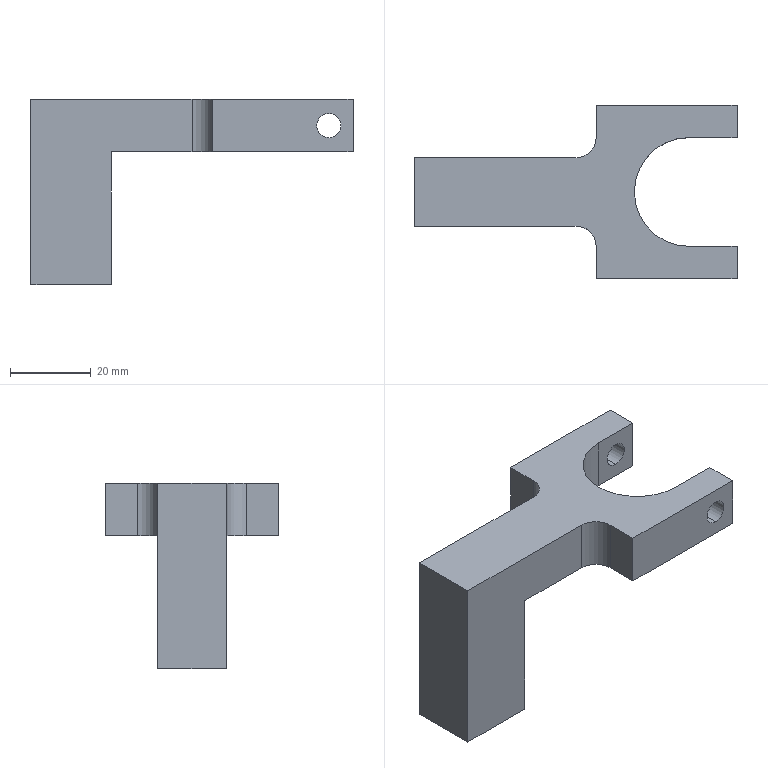Part | SolidWorks | features ICE 3, Extrusion 1, Fillet 1 | 1 solid | 23 faces | box 80 x 43 x 46 mm | volume 32483 mm3 | plane 15 | cylinder 8 | commonest cylinder face diameters 6 x4 10 x2 27 x2
STEP:
#1=CARTESIAN_POINT('',(6.,21.5,-3.));
#2=VERTEX_POINT('',#1);
#3=CARTESIAN_POINT('',(6.,21.5,3.));
#4=VERTEX_POINT('',#3);
#5=CARTESIAN_POINT('',(6.,21.5,0.));
#6=DIRECTION('',(0.,1.,0.));
#7=DIRECTION('',(0.,0.,-1.));
#8=AXIS2_PLACEMENT_3D('',#5,#6,#7);
#9=CIRCLE('',#8,3.);
#10=EDGE_CURVE('',#2,#4,#9,.T.);
#11=ORIENTED_EDGE('',*,*,#10,.T.);
#12=CARTESIAN_POINT('',(6.,13.5,3.));
#13=VERTEX_POINT('',#12);
#14=CARTESIAN_POINT('',(6.,29.985,3.));
#15=DIRECTION('',(0.,-1.,0.));
#16=VECTOR('',#15,1000.);
#17=LINE('',#14,#16);
#18=EDGE_CURVE('',#4,#13,#17,.T.);
#19=ORIENTED_EDGE('',*,*,#18,.T.);
#20=CARTESIAN_POINT('',(6.,13.5,-3.));
#21=VERTEX_POINT('',#20);
#22=CARTESIAN_POINT('',(6.,13.5,0.));
#23=DIRECTION('',(0.,1.,0.));
#24=DIRECTION('',(0.,0.,1.));
#25=AXIS2_PLACEMENT_3D('',#22,#23,#24);
#26=CIRCLE('',#25,3.);
#27=EDGE_CURVE('',#21,#13,#26,.T.);
#28=ORIENTED_EDGE('',*,*,#27,.F.);
#29=CARTESIAN_POINT('',(6.,29.985,-3.));
#30=DIRECTION('',(0.,-1.,0.));
#31=VECTOR('',#30,1000.);
#32=LINE('',#29,#31);
#33=EDGE_CURVE('',#2,#21,#32,.T.);
#34=ORIENTED_EDGE('',*,*,#33,.F.);
#35=EDGE_LOOP('',(#11,#19,#28,#34));
#36=FACE_OUTER_BOUND('',#35,.T.);
#37=CARTESIAN_POINT('',(6.,29.985,0.));
#38=DIRECTION('',(0.,-1.,0.));
#39=DIRECTION('',(0.,0.,-1.));
#40=AXIS2_PLACEMENT_3D('',#37,#38,#39);
#41=CYLINDRICAL_SURFACE('',#40,3.);
#42=ADVANCED_FACE('',(#36),#41,.F.);
#43=CARTESIAN_POINT('',(6.,-13.5,3.));
#44=VERTEX_POINT('',#43);
#45=CARTESIAN_POINT('',(6.,-13.5,-3.));
#46=VERTEX_POINT('',#45);
#47=CARTESIAN_POINT('',(6.,-13.5,0.));
#48=DIRECTION('',(0.,-1.,0.));
#49=DIRECTION('',(0.,0.,-1.));
#50=AXIS2_PLACEMENT_3D('',#47,#48,#49);
#51=CIRCLE('',#50,3.);
#52=EDGE_CURVE('',#44,#46,#51,.T.);
#53=ORIENTED_EDGE('',*,*,#52,.F.);
#54=CARTESIAN_POINT('',(6.,-21.5,3.));
#55=VERTEX_POINT('',#54);
#56=CARTESIAN_POINT('',(6.,29.985,3.));
#57=DIRECTION('',(0.,-1.,0.));
#58=VECTOR('',#57,1000.);
#59=LINE('',#56,#58);
#60=EDGE_CURVE('',#44,#55,#59,.T.);
#61=ORIENTED_EDGE('',*,*,#60,.T.);
#62=CARTESIAN_POINT('',(6.,-21.5,-3.));
#63=VERTEX_POINT('',#62);
#64=CARTESIAN_POINT('',(6.,-21.5,0.));
#65=DIRECTION('',(0.,-1.,0.));
#66=DIRECTION('',(0.,0.,-1.));
#67=AXIS2_PLACEMENT_3D('',#64,#65,#66);
#68=CIRCLE('',#67,3.);
#69=EDGE_CURVE('',#55,#63,#68,.T.);
#70=ORIENTED_EDGE('',*,*,#69,.T.);
#71=CARTESIAN_POINT('',(6.,29.985,-3.));
#72=DIRECTION('',(0.,-1.,0.));
#73=VECTOR('',#72,1000.);
#74=LINE('',#71,#73);
#75=EDGE_CURVE('',#46,#63,#74,.T.);
#76=ORIENTED_EDGE('',*,*,#75,.F.);
#77=EDGE_LOOP('',(#53,#61,#70,#76));
#78=FACE_OUTER_BOUND('',#77,.T.);
#79=CARTESIAN_POINT('',(6.,29.985,0.));
#80=DIRECTION('',(0.,-1.,0.));
#81=DIRECTION('',(0.,0.,-1.));
#82=AXIS2_PLACEMENT_3D('',#79,#80,#81);
#83=CYLINDRICAL_SURFACE('',#82,3.);
#84=ADVANCED_FACE('',(#78),#83,.F.);
#85=CARTESIAN_POINT('',(-13.5,0.,6.5));
#86=VERTEX_POINT('',#85);
#87=CARTESIAN_POINT('',(0.,13.5,6.5));
#88=VERTEX_POINT('',#87);
#89=CARTESIAN_POINT('',(0.,0.,6.5));
#90=DIRECTION('',(0.,0.,-1.));
#91=DIRECTION('',(1.,0.,0.));
#92=AXIS2_PLACEMENT_3D('',#89,#90,#91);
#93=CIRCLE('',#92,13.5);
#94=EDGE_CURVE('',#86,#88,#93,.T.);
#95=ORIENTED_EDGE('',*,*,#94,.F.);
#96=CARTESIAN_POINT('',(-13.5,0.,-6.5));
#97=VERTEX_POINT('',#96);
#98=CARTESIAN_POINT('',(-13.5,0.,6.5));
#99=DIRECTION('',(0.,0.,-1.));
#100=VECTOR('',#99,1000.);
#101=LINE('',#98,#100);
#102=EDGE_CURVE('',#86,#97,#101,.T.);
#103=ORIENTED_EDGE('',*,*,#102,.T.);
#104=CARTESIAN_POINT('',(0.,13.5,-6.5));
#105=VERTEX_POINT('',#104);
#106=CARTESIAN_POINT('',(0.,0.,-6.5));
#107=DIRECTION('',(0.,0.,-1.));
#108=DIRECTION('',(1.,0.,0.));
#109=AXIS2_PLACEMENT_3D('',#106,#107,#108);
#110=CIRCLE('',#109,13.5);
#111=EDGE_CURVE('',#97,#105,#110,.T.);
#112=ORIENTED_EDGE('',*,*,#111,.T.);
#113=CARTESIAN_POINT('',(0.,13.5,6.5));
#114=DIRECTION('',(0.,0.,-1.));
#115=VECTOR('',#114,1000.);
#116=LINE('',#113,#115);
#117=EDGE_CURVE('',#88,#105,#116,.T.);
#118=ORIENTED_EDGE('',*,*,#117,.F.);
#119=EDGE_LOOP('',(#95,#103,#112,#118));
#120=FACE_OUTER_BOUND('',#119,.T.);
#121=CARTESIAN_POINT('',(0.,0.,6.5));
#122=DIRECTION('',(0.,0.,-1.));
#123=DIRECTION('',(-1.,0.,0.));
#124=AXIS2_PLACEMENT_3D('',#121,#122,#123);
#125=CYLINDRICAL_SURFACE('',#124,13.5);
#126=ADVANCED_FACE('',(#120),#125,.F.);
#127=CARTESIAN_POINT('',(-48.,8.5,-6.5));
#128=VERTEX_POINT('',#127);
#129=CARTESIAN_POINT('',(-48.,-8.5,-6.5));
#130=VERTEX_POINT('',#129);
#131=CARTESIAN_POINT('',(-48.,-8.5,-6.5));
#132=DIRECTION('',(0.,-1.,0.));
#133=VECTOR('',#132,1000.);
#134=LINE('',#131,#133);
#135=EDGE_CURVE('',#128,#130,#134,.T.);
#136=ORIENTED_EDGE('',*,*,#135,.F.);
#137=CARTESIAN_POINT('',(-28.,8.5,-6.5));
#138=VERTEX_POINT('',#137);
#139=CARTESIAN_POINT('',(-68.,8.5,-6.5));
#140=DIRECTION('',(-1.,0.,0.));
#141=VECTOR('',#140,1000.);
#142=LINE('',#139,#141);
#143=EDGE_CURVE('',#138,#128,#142,.T.);
#144=ORIENTED_EDGE('',*,*,#143,.F.);
#145=CARTESIAN_POINT('',(-23.,13.5,-6.5));
#146=VERTEX_POINT('',#145);
#147=CARTESIAN_POINT('',(-28.,13.5,-6.5));
#148=DIRECTION('',(0.,0.,1.));
#149=DIRECTION('',(1.,0.,0.));
#150=AXIS2_PLACEMENT_3D('',#147,#148,#149);
#151=CIRCLE('',#150,5.);
#152=EDGE_CURVE('',#138,#146,#151,.T.);
#153=ORIENTED_EDGE('',*,*,#152,.T.);
#154=CARTESIAN_POINT('',(-23.,21.5,-6.5));
#155=VERTEX_POINT('',#154);
#156=CARTESIAN_POINT('',(-23.,21.5,-6.5));
#157=DIRECTION('',(0.,-1.,0.));
#158=VECTOR('',#157,1000.);
#159=LINE('',#156,#158);
#160=EDGE_CURVE('',#155,#146,#159,.T.);
#161=ORIENTED_EDGE('',*,*,#160,.F.);
#162=CARTESIAN_POINT('',(12.,21.5,-6.5));
#163=VERTEX_POINT('',#162);
#164=CARTESIAN_POINT('',(12.,21.5,-6.5));
#165=DIRECTION('',(-1.,0.,0.));
#166=VECTOR('',#165,1000.);
#167=LINE('',#164,#166);
#168=EDGE_CURVE('',#163,#155,#167,.T.);
#169=ORIENTED_EDGE('',*,*,#168,.F.);
#170=CARTESIAN_POINT('',(12.,13.5,-6.5));
#171=VERTEX_POINT('',#170);
#172=CARTESIAN_POINT('',(12.,13.5,-6.5));
#173=DIRECTION('',(0.,1.,0.));
#174=VECTOR('',#173,1000.);
#175=LINE('',#172,#174);
#176=EDGE_CURVE('',#171,#163,#175,.T.);
#177=ORIENTED_EDGE('',*,*,#176,.F.);
#178=CARTESIAN_POINT('',(0.,13.5,-6.5));
#179=DIRECTION('',(1.,0.,0.));
#180=VECTOR('',#179,1000.);
#181=LINE('',#178,#180);
#182=EDGE_CURVE('',#105,#171,#181,.T.);
#183=ORIENTED_EDGE('',*,*,#182,.F.);
#184=ORIENTED_EDGE('',*,*,#111,.F.);
#185=CARTESIAN_POINT('',(0.,-13.5,-6.5));
#186=VERTEX_POINT('',#185);
#187=CARTESIAN_POINT('',(0.,0.,-6.5));
#188=DIRECTION('',(0.,0.,-1.));
#189=DIRECTION('',(1.,0.,0.));
#190=AXIS2_PLACEMENT_3D('',#187,#188,#189);
#191=CIRCLE('',#190,13.5);
#192=EDGE_CURVE('',#186,#97,#191,.T.);
#193=ORIENTED_EDGE('',*,*,#192,.F.);
#194=CARTESIAN_POINT('',(12.,-13.5,-6.5));
#195=VERTEX_POINT('',#194);
#196=CARTESIAN_POINT('',(12.,-13.5,-6.5));
#197=DIRECTION('',(-1.,0.,0.));
#198=VECTOR('',#197,1000.);
#199=LINE('',#196,#198);
#200=EDGE_CURVE('',#195,#186,#199,.T.);
#201=ORIENTED_EDGE('',*,*,#200,.F.);
#202=CARTESIAN_POINT('',(12.,-21.5,-6.5));
#203=VERTEX_POINT('',#202);
#204=CARTESIAN_POINT('',(12.,-21.5,-6.5));
#205=DIRECTION('',(0.,1.,0.));
#206=VECTOR('',#205,1000.);
#207=LINE('',#204,#206);
#208=EDGE_CURVE('',#203,#195,#207,.T.);
#209=ORIENTED_EDGE('',*,*,#208,.F.);
#210=CARTESIAN_POINT('',(-23.,-21.5,-6.5));
#211=VERTEX_POINT('',#210);
#212=CARTESIAN_POINT('',(-68.,-21.5,-6.5));
#213=DIRECTION('',(1.,0.,0.));
#214=VECTOR('',#213,1000.);
#215=LINE('',#212,#214);
#216=EDGE_CURVE('',#211,#203,#215,.T.);
#217=ORIENTED_EDGE('',*,*,#216,.F.);
#218=CARTESIAN_POINT('',(-23.,-13.5,-6.5));
#219=VERTEX_POINT('',#218);
#220=CARTESIAN_POINT('',(-23.,-21.5,-6.5));
#221=DIRECTION('',(0.,-1.,0.));
#222=VECTOR('',#221,1000.);
#223=LINE('',#220,#222);
#224=EDGE_CURVE('',#219,#211,#223,.T.);
#225=ORIENTED_EDGE('',*,*,#224,.F.);
#226=CARTESIAN_POINT('',(-28.,-8.5,-6.5));
#227=VERTEX_POINT('',#226);
#228=CARTESIAN_POINT('',(-28.,-13.5,-6.5));
#229=DIRECTION('',(0.,0.,1.));
#230=DIRECTION('',(1.,0.,0.));
#231=AXIS2_PLACEMENT_3D('',#228,#229,#230);
#232=CIRCLE('',#231,5.);
#233=EDGE_CURVE('',#219,#227,#232,.T.);
#234=ORIENTED_EDGE('',*,*,#233,.T.);
#235=CARTESIAN_POINT('',(-68.,-8.5,-6.5));
#236=DIRECTION('',(1.,0.,0.));
#237=VECTOR('',#236,1000.);
#238=LINE('',#235,#237);
#239=EDGE_CURVE('',#130,#227,#238,.T.);
#240=ORIENTED_EDGE('',*,*,#239,.F.);
#241=EDGE_LOOP('',(#136,#144,#153,#161,#169,#177,#183,#184,#193,#201,#209,#217,#225,#234,#240));
#242=FACE_OUTER_BOUND('',#241,.T.);
#243=CARTESIAN_POINT('',(0.,0.,-6.5));
#244=DIRECTION('',(0.,0.,1.));
#245=DIRECTION('',(1.,0.,0.));
#246=AXIS2_PLACEMENT_3D('',#243,#244,#245);
#247=PLANE('',#246);
#248=ADVANCED_FACE('',(#242),#247,.F.);
#249=ORIENTED_EDGE('',*,*,#102,.F.);
#250=CARTESIAN_POINT('',(0.,-13.5,6.5));
#251=VERTEX_POINT('',#250);
#252=CARTESIAN_POINT('',(0.,0.,6.5));
#253=DIRECTION('',(0.,0.,-1.));
#254=DIRECTION('',(1.,0.,0.));
#255=AXIS2_PLACEMENT_3D('',#252,#253,#254);
#256=CIRCLE('',#255,13.5);
#257=EDGE_CURVE('',#251,#86,#256,.T.);
#258=ORIENTED_EDGE('',*,*,#257,.F.);
#259=CARTESIAN_POINT('',(0.,-13.5,6.5));
#260=DIRECTION('',(0.,0.,-1.));
#261=VECTOR('',#260,1000.);
#262=LINE('',#259,#261);
#263=EDGE_CURVE('',#251,#186,#262,.T.);
#264=ORIENTED_EDGE('',*,*,#263,.T.);
#265=ORIENTED_EDGE('',*,*,#192,.T.);
#266=EDGE_LOOP('',(#249,#258,#264,#265));
#267=FACE_OUTER_BOUND('',#266,.T.);
#268=CARTESIAN_POINT('',(0.,0.,6.5));
#269=DIRECTION('',(0.,0.,-1.));
#270=DIRECTION('',(-1.,0.,0.));
#271=AXIS2_PLACEMENT_3D('',#268,#269,#270);
#272=CYLINDRICAL_SURFACE('',#271,13.5);
#273=ADVANCED_FACE('',(#267),#272,.F.);
#274=ORIENTED_EDGE('',*,*,#27,.T.);
#275=CARTESIAN_POINT('',(6.,13.5,0.));
#276=DIRECTION('',(0.,1.,0.));
#277=DIRECTION('',(0.,0.,1.));
#278=AXIS2_PLACEMENT_3D('',#275,#276,#277);
#279=CIRCLE('',#278,3.);
#280=EDGE_CURVE('',#13,#21,#279,.T.);
#281=ORIENTED_EDGE('',*,*,#280,.T.);
#282=EDGE_LOOP('',(#274,#281));
#283=FACE_BOUND('',#282,.T.);
#284=ORIENTED_EDGE('',*,*,#182,.T.);
#285=CARTESIAN_POINT('',(12.,13.5,6.5));
#286=VERTEX_POINT('',#285);
#287=CARTESIAN_POINT('',(12.,13.5,6.5));
#288=DIRECTION('',(0.,0.,-1.));
#289=VECTOR('',#288,1000.);
#290=LINE('',#287,#289);
#291=EDGE_CURVE('',#286,#171,#290,.T.);
#292=ORIENTED_EDGE('',*,*,#291,.F.);
#293=CARTESIAN_POINT('',(0.,13.5,6.5));
#294=DIRECTION('',(1.,0.,0.));
#295=VECTOR('',#294,1000.);
#296=LINE('',#293,#295);
#297=EDGE_CURVE('',#88,#286,#296,.T.);
#298=ORIENTED_EDGE('',*,*,#297,.F.);
#299=ORIENTED_EDGE('',*,*,#117,.T.);
#300=EDGE_LOOP('',(#284,#292,#298,#299));
#301=FACE_OUTER_BOUND('',#300,.T.);
#302=CARTESIAN_POINT('',(0.,13.5,6.5));
#303=DIRECTION('',(0.,1.,0.));
#304=DIRECTION('',(0.,0.,1.));
#305=AXIS2_PLACEMENT_3D('',#302,#303,#304);
#306=PLANE('',#305);
#307=ADVANCED_FACE('',(#283,#301),#306,.F.);
#308=ORIENTED_EDGE('',*,*,#176,.T.);
#309=CARTESIAN_POINT('',(12.,21.5,6.5));
#310=VERTEX_POINT('',#309);
#311=CARTESIAN_POINT('',(12.,21.5,6.5));
#312=DIRECTION('',(0.,0.,-1.));
#313=VECTOR('',#312,1000.);
#314=LINE('',#311,#313);
#315=EDGE_CURVE('',#310,#163,#314,.T.);
#316=ORIENTED_EDGE('',*,*,#315,.F.);
#317=CARTESIAN_POINT('',(12.,13.5,6.5));
#318=DIRECTION('',(0.,1.,0.));
#319=VECTOR('',#318,1000.);
#320=LINE('',#317,#319);
#321=EDGE_CURVE('',#286,#310,#320,.T.);
#322=ORIENTED_EDGE('',*,*,#321,.F.);
#323=ORIENTED_EDGE('',*,*,#291,.T.);
#324=EDGE_LOOP('',(#308,#316,#322,#323));
#325=FACE_OUTER_BOUND('',#324,.T.);
#326=CARTESIAN_POINT('',(12.,13.5,6.5));
#327=DIRECTION('',(-1.,0.,0.));
#328=DIRECTION('',(0.,0.,1.));
#329=AXIS2_PLACEMENT_3D('',#326,#327,#328);
#330=PLANE('',#329);
#331=ADVANCED_FACE('',(#325),#330,.F.);
#332=ORIENTED_EDGE('',*,*,#10,.F.);
#333=CARTESIAN_POINT('',(6.,21.5,0.));
#334=DIRECTION('',(0.,1.,0.));
#335=DIRECTION('',(0.,0.,-1.));
#336=AXIS2_PLACEMENT_3D('',#333,#334,#335);
#337=CIRCLE('',#336,3.);
#338=EDGE_CURVE('',#4,#2,#337,.T.);
#339=ORIENTED_EDGE('',*,*,#338,.F.);
#340=EDGE_LOOP('',(#332,#339));
#341=FACE_BOUND('',#340,.T.);
#342=ORIENTED_EDGE('',*,*,#168,.T.);
#343=CARTESIAN_POINT('',(-23.,21.5,6.5));
#344=VERTEX_POINT('',#343);
#345=CARTESIAN_POINT('',(-23.,21.5,-6.501));
#346=DIRECTION('',(0.,0.,1.));
#347=VECTOR('',#346,1000.);
#348=LINE('',#345,#347);
#349=EDGE_CURVE('',#155,#344,#348,.T.);
#350=ORIENTED_EDGE('',*,*,#349,.T.);
#351=CARTESIAN_POINT('',(12.,21.5,6.5));
#352=DIRECTION('',(-1.,0.,0.));
#353=VECTOR('',#352,1000.);
#354=LINE('',#351,#353);
#355=EDGE_CURVE('',#310,#344,#354,.T.);
#356=ORIENTED_EDGE('',*,*,#355,.F.);
#357=ORIENTED_EDGE('',*,*,#315,.T.);
#358=EDGE_LOOP('',(#342,#350,#356,#357));
#359=FACE_OUTER_BOUND('',#358,.T.);
#360=CARTESIAN_POINT('',(12.,21.5,6.5));
#361=DIRECTION('',(0.,-1.,0.));
#362=DIRECTION('',(0.,0.,-1.));
#363=AXIS2_PLACEMENT_3D('',#360,#361,#362);
#364=PLANE('',#363);
#365=ADVANCED_FACE('',(#341,#359),#364,.F.);
#366=CARTESIAN_POINT('',(-68.,8.5,6.5));
#367=VERTEX_POINT('',#366);
#368=CARTESIAN_POINT('',(-68.,-8.5,6.5));
#369=VERTEX_POINT('',#368);
#370=CARTESIAN_POINT('',(-68.,21.5,6.5));
#371=DIRECTION('',(0.,-1.,0.));
#372=VECTOR('',#371,1000.);
#373=LINE('',#370,#372);
#374=EDGE_CURVE('',#367,#369,#373,.T.);
#375=ORIENTED_EDGE('',*,*,#374,.F.);
#376=CARTESIAN_POINT('',(-68.,8.5,-39.5));
#377=VERTEX_POINT('',#376);
#378=CARTESIAN_POINT('',(-68.,8.5,-6.501));
#379=DIRECTION('',(0.,0.,1.));
#380=VECTOR('',#379,1000.);
#381=LINE('',#378,#380);
#382=EDGE_CURVE('',#377,#367,#381,.T.);
#383=ORIENTED_EDGE('',*,*,#382,.F.);
#384=CARTESIAN_POINT('',(-68.,-8.5,-39.5));
#385=VERTEX_POINT('',#384);
#386=CARTESIAN_POINT('',(-68.,-8.5,-39.5));
#387=DIRECTION('',(0.,1.,0.));
#388=VECTOR('',#387,1000.);
#389=LINE('',#386,#388);
#390=EDGE_CURVE('',#385,#377,#389,.T.);
#391=ORIENTED_EDGE('',*,*,#390,.F.);
#392=CARTESIAN_POINT('',(-68.,-8.5,-6.501));
#393=DIRECTION('',(0.,0.,1.));
#394=VECTOR('',#393,1000.);
#395=LINE('',#392,#394);
#396=EDGE_CURVE('',#385,#369,#395,.T.);
#397=ORIENTED_EDGE('',*,*,#396,.T.);
#398=EDGE_LOOP('',(#375,#383,#391,#397));
#399=FACE_OUTER_BOUND('',#398,.T.);
#400=CARTESIAN_POINT('',(-68.,21.5,6.5));
#401=DIRECTION('',(1.,0.,0.));
#402=DIRECTION('',(0.,0.,-1.));
#403=AXIS2_PLACEMENT_3D('',#400,#401,#402);
#404=PLANE('',#403);
#405=ADVANCED_FACE('',(#399),#404,.F.);
#406=CARTESIAN_POINT('',(6.,-21.5,0.));
#407=DIRECTION('',(0.,-1.,0.));
#408=DIRECTION('',(0.,0.,-1.));
#409=AXIS2_PLACEMENT_3D('',#406,#407,#408);
#410=CIRCLE('',#409,3.);
#411=EDGE_CURVE('',#63,#55,#410,.T.);
#412=ORIENTED_EDGE('',*,*,#411,.F.);
#413=ORIENTED_EDGE('',*,*,#69,.F.);
#414=EDGE_LOOP('',(#412,#413));
#415=FACE_BOUND('',#414,.T.);
#416=CARTESIAN_POINT('',(-23.,-21.5,6.5));
#417=VERTEX_POINT('',#416);
#418=CARTESIAN_POINT('',(12.,-21.5,6.5));
#419=VERTEX_POINT('',#418);
#420=CARTESIAN_POINT('',(-68.,-21.5,6.5));
#421=DIRECTION('',(1.,0.,0.));
#422=VECTOR('',#421,1000.);
#423=LINE('',#420,#422);
#424=EDGE_CURVE('',#417,#419,#423,.T.);
#425=ORIENTED_EDGE('',*,*,#424,.F.);
#426=CARTESIAN_POINT('',(-23.,-21.5,-6.501));
#427=DIRECTION('',(0.,0.,1.));
#428=VECTOR('',#427,1000.);
#429=LINE('',#426,#428);
#430=EDGE_CURVE('',#211,#417,#429,.T.);
#431=ORIENTED_EDGE('',*,*,#430,.F.);
#432=ORIENTED_EDGE('',*,*,#216,.T.);
#433=CARTESIAN_POINT('',(12.,-21.5,6.5));
#434=DIRECTION('',(0.,0.,-1.));
#435=VECTOR('',#434,1000.);
#436=LINE('',#433,#435);
#437=EDGE_CURVE('',#419,#203,#436,.T.);
#438=ORIENTED_EDGE('',*,*,#437,.F.);
#439=EDGE_LOOP('',(#425,#431,#432,#438));
#440=FACE_OUTER_BOUND('',#439,.T.);
#441=CARTESIAN_POINT('',(-68.,-21.5,6.5));
#442=DIRECTION('',(0.,1.,0.));
#443=DIRECTION('',(0.,0.,1.));
#444=AXIS2_PLACEMENT_3D('',#441,#442,#443);
#445=PLANE('',#444);
#446=ADVANCED_FACE('',(#415,#440),#445,.F.);
#447=ORIENTED_EDGE('',*,*,#208,.T.);
#448=CARTESIAN_POINT('',(12.,-13.5,6.5));
#449=VERTEX_POINT('',#448);
#450=CARTESIAN_POINT('',(12.,-13.5,6.5));
#451=DIRECTION('',(0.,0.,-1.));
#452=VECTOR('',#451,1000.);
#453=LINE('',#450,#452);
#454=EDGE_CURVE('',#449,#195,#453,.T.);
#455=ORIENTED_EDGE('',*,*,#454,.F.);
#456=CARTESIAN_POINT('',(12.,-21.5,6.5));
#457=DIRECTION('',(0.,1.,0.));
#458=VECTOR('',#457,1000.);
#459=LINE('',#456,#458);
#460=EDGE_CURVE('',#419,#449,#459,.T.);
#461=ORIENTED_EDGE('',*,*,#460,.F.);
#462=ORIENTED_EDGE('',*,*,#437,.T.);
#463=EDGE_LOOP('',(#447,#455,#461,#462));
#464=FACE_OUTER_BOUND('',#463,.T.);
#465=CARTESIAN_POINT('',(12.,-21.5,6.5));
#466=DIRECTION('',(-1.,0.,0.));
#467=DIRECTION('',(0.,0.,1.));
#468=AXIS2_PLACEMENT_3D('',#465,#466,#467);
#469=PLANE('',#468);
#470=ADVANCED_FACE('',(#464),#469,.F.);
#471=CARTESIAN_POINT('',(6.,-13.5,0.));
#472=DIRECTION('',(0.,-1.,0.));
#473=DIRECTION('',(0.,0.,-1.));
#474=AXIS2_PLACEMENT_3D('',#471,#472,#473);
#475=CIRCLE('',#474,3.);
#476=EDGE_CURVE('',#46,#44,#475,.T.);
#477=ORIENTED_EDGE('',*,*,#476,.T.);
#478=ORIENTED_EDGE('',*,*,#52,.T.);
#479=EDGE_LOOP('',(#477,#478));
#480=FACE_BOUND('',#479,.T.);
#481=ORIENTED_EDGE('',*,*,#200,.T.);
#482=ORIENTED_EDGE('',*,*,#263,.F.);
#483=CARTESIAN_POINT('',(12.,-13.5,6.5));
#484=DIRECTION('',(-1.,0.,0.));
#485=VECTOR('',#484,1000.);
#486=LINE('',#483,#485);
#487=EDGE_CURVE('',#449,#251,#486,.T.);
#488=ORIENTED_EDGE('',*,*,#487,.F.);
#489=ORIENTED_EDGE('',*,*,#454,.T.);
#490=EDGE_LOOP('',(#481,#482,#488,#489));
#491=FACE_OUTER_BOUND('',#490,.T.);
#492=CARTESIAN_POINT('',(12.,-13.5,6.5));
#493=DIRECTION('',(0.,-1.,0.));
#494=DIRECTION('',(0.,0.,-1.));
#495=AXIS2_PLACEMENT_3D('',#492,#493,#494);
#496=PLANE('',#495);
#497=ADVANCED_FACE('',(#480,#491),#496,.F.);
#498=CARTESIAN_POINT('',(-23.,13.5,6.5));
#499=VERTEX_POINT('',#498);
#500=CARTESIAN_POINT('',(-23.,21.5,6.5));
#501=DIRECTION('',(0.,1.,0.));
#502=VECTOR('',#501,1000.);
#503=LINE('',#500,#502);
#504=EDGE_CURVE('',#499,#344,#503,.T.);
#505=ORIENTED_EDGE('',*,*,#504,.F.);
#506=CARTESIAN_POINT('',(-28.,8.5,6.5));
#507=VERTEX_POINT('',#506);
#508=CARTESIAN_POINT('',(-28.,13.5,6.5));
#509=DIRECTION('',(0.,0.,-1.));
#510=DIRECTION('',(1.,0.,0.));
#511=AXIS2_PLACEMENT_3D('',#508,#509,#510);
#512=CIRCLE('',#511,5.);
#513=EDGE_CURVE('',#499,#507,#512,.T.);
#514=ORIENTED_EDGE('',*,*,#513,.T.);
#515=CARTESIAN_POINT('',(-68.,8.5,6.5));
#516=DIRECTION('',(1.,0.,0.));
#517=VECTOR('',#516,1000.);
#518=LINE('',#515,#517);
#519=EDGE_CURVE('',#367,#507,#518,.T.);
#520=ORIENTED_EDGE('',*,*,#519,.F.);
#521=ORIENTED_EDGE('',*,*,#374,.T.);
#522=CARTESIAN_POINT('',(-28.,-8.5,6.5));
#523=VERTEX_POINT('',#522);
#524=CARTESIAN_POINT('',(-68.,-8.5,6.5));
#525=DIRECTION('',(-1.,0.,0.));
#526=VECTOR('',#525,1000.);
#527=LINE('',#524,#526);
#528=EDGE_CURVE('',#523,#369,#527,.T.);
#529=ORIENTED_EDGE('',*,*,#528,.F.);
#530=CARTESIAN_POINT('',(-23.,-13.5,6.5));
#531=VERTEX_POINT('',#530);
#532=CARTESIAN_POINT('',(-28.,-13.5,6.5));
#533=DIRECTION('',(0.,0.,-1.));
#534=DIRECTION('',(1.,0.,0.));
#535=AXIS2_PLACEMENT_3D('',#532,#533,#534);
#536=CIRCLE('',#535,5.);
#537=EDGE_CURVE('',#523,#531,#536,.T.);
#538=ORIENTED_EDGE('',*,*,#537,.T.);
#539=CARTESIAN_POINT('',(-23.,-21.5,6.5));
#540=DIRECTION('',(0.,1.,0.));
#541=VECTOR('',#540,1000.);
#542=LINE('',#539,#541);
#543=EDGE_CURVE('',#417,#531,#542,.T.);
#544=ORIENTED_EDGE('',*,*,#543,.F.);
#545=ORIENTED_EDGE('',*,*,#424,.T.);
#546=ORIENTED_EDGE('',*,*,#460,.T.);
#547=ORIENTED_EDGE('',*,*,#487,.T.);
#548=ORIENTED_EDGE('',*,*,#257,.T.);
#549=ORIENTED_EDGE('',*,*,#94,.T.);
#550=ORIENTED_EDGE('',*,*,#297,.T.);
#551=ORIENTED_EDGE('',*,*,#321,.T.);
#552=ORIENTED_EDGE('',*,*,#355,.T.);
#553=EDGE_LOOP('',(#505,#514,#520,#521,#529,#538,#544,#545,#546,#547,#548,#549,#550,#551,#552));
#554=FACE_OUTER_BOUND('',#553,.T.);
#555=CARTESIAN_POINT('',(0.,0.,6.5));
#556=DIRECTION('',(0.,0.,1.));
#557=DIRECTION('',(1.,0.,0.));
#558=AXIS2_PLACEMENT_3D('',#555,#556,#557);
#559=PLANE('',#558);
#560=ADVANCED_FACE('',(#554),#559,.T.);
#561=ORIENTED_EDGE('',*,*,#396,.F.);
#562=CARTESIAN_POINT('',(-48.,-8.5,-39.5));
#563=VERTEX_POINT('',#562);
#564=CARTESIAN_POINT('',(-68.,-8.5,-39.5));
#565=DIRECTION('',(-1.,0.,0.));
#566=VECTOR('',#565,1000.);
#567=LINE('',#564,#566);
#568=EDGE_CURVE('',#563,#385,#567,.T.);
#569=ORIENTED_EDGE('',*,*,#568,.F.);
#570=CARTESIAN_POINT('',(-48.,-8.5,-39.5));
#571=DIRECTION('',(0.,0.,1.));
#572=VECTOR('',#571,1000.);
#573=LINE('',#570,#572);
#574=EDGE_CURVE('',#563,#130,#573,.T.);
#575=ORIENTED_EDGE('',*,*,#574,.T.);
#576=ORIENTED_EDGE('',*,*,#239,.T.);
#577=CARTESIAN_POINT('',(-28.,-8.5,6.5));
#578=DIRECTION('',(0.,0.,1.));
#579=VECTOR('',#578,1000.);
#580=LINE('',#577,#579);
#581=EDGE_CURVE('',#227,#523,#580,.T.);
#582=ORIENTED_EDGE('',*,*,#581,.T.);
#583=ORIENTED_EDGE('',*,*,#528,.T.);
#584=EDGE_LOOP('',(#561,#569,#575,#576,#582,#583));
#585=FACE_OUTER_BOUND('',#584,.T.);
#586=CARTESIAN_POINT('',(-68.,-8.5,-6.501));
#587=DIRECTION('',(0.,1.,0.));
#588=DIRECTION('',(0.,0.,1.));
#589=AXIS2_PLACEMENT_3D('',#586,#587,#588);
#590=PLANE('',#589);
#591=ADVANCED_FACE('',(#585),#590,.F.);
#592=ORIENTED_EDGE('',*,*,#543,.T.);
#593=CARTESIAN_POINT('',(-23.,-13.5,-6.5));
#594=DIRECTION('',(0.,0.,-1.));
#595=VECTOR('',#594,1000.);
#596=LINE('',#593,#595);
#597=EDGE_CURVE('',#531,#219,#596,.T.);
#598=ORIENTED_EDGE('',*,*,#597,.T.);
#599=ORIENTED_EDGE('',*,*,#224,.T.);
#600=ORIENTED_EDGE('',*,*,#430,.T.);
#601=EDGE_LOOP('',(#592,#598,#599,#600));
#602=FACE_OUTER_BOUND('',#601,.T.);
#603=CARTESIAN_POINT('',(-23.,-21.5,-6.501));
#604=DIRECTION('',(1.,0.,0.));
#605=DIRECTION('',(0.,0.,-1.));
#606=AXIS2_PLACEMENT_3D('',#603,#604,#605);
#607=PLANE('',#606);
#608=ADVANCED_FACE('',(#602),#607,.F.);
#609=ORIENTED_EDGE('',*,*,#160,.T.);
#610=CARTESIAN_POINT('',(-23.,13.5,6.5));
#611=DIRECTION('',(0.,0.,1.));
#612=VECTOR('',#611,1000.);
#613=LINE('',#610,#612);
#614=EDGE_CURVE('',#146,#499,#613,.T.);
#615=ORIENTED_EDGE('',*,*,#614,.T.);
#616=ORIENTED_EDGE('',*,*,#504,.T.);
#617=ORIENTED_EDGE('',*,*,#349,.F.);
#618=EDGE_LOOP('',(#609,#615,#616,#617));
#619=FACE_OUTER_BOUND('',#618,.T.);
#620=CARTESIAN_POINT('',(-23.,21.5,-6.501));
#621=DIRECTION('',(1.,0.,0.));
#622=DIRECTION('',(0.,0.,-1.));
#623=AXIS2_PLACEMENT_3D('',#620,#621,#622);
#624=PLANE('',#623);
#625=ADVANCED_FACE('',(#619),#624,.F.);
#626=ORIENTED_EDGE('',*,*,#519,.T.);
#627=CARTESIAN_POINT('',(-28.,8.5,-6.5));
#628=DIRECTION('',(0.,0.,-1.));
#629=VECTOR('',#628,1000.);
#630=LINE('',#627,#629);
#631=EDGE_CURVE('',#507,#138,#630,.T.);
#632=ORIENTED_EDGE('',*,*,#631,.T.);
#633=ORIENTED_EDGE('',*,*,#143,.T.);
#634=CARTESIAN_POINT('',(-48.,8.5,-39.5));
#635=VERTEX_POINT('',#634);
#636=CARTESIAN_POINT('',(-48.,8.5,-39.5));
#637=DIRECTION('',(0.,0.,1.));
#638=VECTOR('',#637,1000.);
#639=LINE('',#636,#638);
#640=EDGE_CURVE('',#635,#128,#639,.T.);
#641=ORIENTED_EDGE('',*,*,#640,.F.);
#642=CARTESIAN_POINT('',(-68.,8.5,-39.5));
#643=DIRECTION('',(1.,0.,0.));
#644=VECTOR('',#643,1000.);
#645=LINE('',#642,#644);
#646=EDGE_CURVE('',#377,#635,#645,.T.);
#647=ORIENTED_EDGE('',*,*,#646,.F.);
#648=ORIENTED_EDGE('',*,*,#382,.T.);
#649=EDGE_LOOP('',(#626,#632,#633,#641,#647,#648));
#650=FACE_OUTER_BOUND('',#649,.T.);
#651=CARTESIAN_POINT('',(-68.,8.5,-6.501));
#652=DIRECTION('',(0.,-1.,0.));
#653=DIRECTION('',(0.,0.,-1.));
#654=AXIS2_PLACEMENT_3D('',#651,#652,#653);
#655=PLANE('',#654);
#656=ADVANCED_FACE('',(#650),#655,.F.);
#657=ORIENTED_EDGE('',*,*,#233,.F.);
#658=ORIENTED_EDGE('',*,*,#597,.F.);
#659=ORIENTED_EDGE('',*,*,#537,.F.);
#660=ORIENTED_EDGE('',*,*,#581,.F.);
#661=EDGE_LOOP('',(#657,#658,#659,#660));
#662=FACE_OUTER_BOUND('',#661,.T.);
#663=CARTESIAN_POINT('',(-28.,-13.5,-6.501));
#664=DIRECTION('',(0.,0.,-1.));
#665=DIRECTION('',(-1.,0.,0.));
#666=AXIS2_PLACEMENT_3D('',#663,#664,#665);
#667=CYLINDRICAL_SURFACE('',#666,5.);
#668=ADVANCED_FACE('',(#662),#667,.F.);
#669=ORIENTED_EDGE('',*,*,#152,.F.);
#670=ORIENTED_EDGE('',*,*,#631,.F.);
#671=ORIENTED_EDGE('',*,*,#513,.F.);
#672=ORIENTED_EDGE('',*,*,#614,.F.);
#673=EDGE_LOOP('',(#669,#670,#671,#672));
#674=FACE_OUTER_BOUND('',#673,.T.);
#675=CARTESIAN_POINT('',(-28.,13.5,-6.501));
#676=DIRECTION('',(0.,0.,-1.));
#677=DIRECTION('',(-1.,0.,0.));
#678=AXIS2_PLACEMENT_3D('',#675,#676,#677);
#679=CYLINDRICAL_SURFACE('',#678,5.);
#680=ADVANCED_FACE('',(#674),#679,.F.);
#681=ORIENTED_EDGE('',*,*,#135,.T.);
#682=ORIENTED_EDGE('',*,*,#574,.F.);
#683=CARTESIAN_POINT('',(-48.,-8.5,-39.5));
#684=DIRECTION('',(0.,-1.,0.));
#685=VECTOR('',#684,1000.);
#686=LINE('',#683,#685);
#687=EDGE_CURVE('',#635,#563,#686,.T.);
#688=ORIENTED_EDGE('',*,*,#687,.F.);
#689=ORIENTED_EDGE('',*,*,#640,.T.);
#690=EDGE_LOOP('',(#681,#682,#688,#689));
#691=FACE_OUTER_BOUND('',#690,.T.);
#692=CARTESIAN_POINT('',(-48.,-8.5,-39.5));
#693=DIRECTION('',(-1.,0.,0.));
#694=DIRECTION('',(0.,0.,1.));
#695=AXIS2_PLACEMENT_3D('',#692,#693,#694);
#696=PLANE('',#695);
#697=ADVANCED_FACE('',(#691),#696,.F.);
#698=ORIENTED_EDGE('',*,*,#390,.T.);
#699=ORIENTED_EDGE('',*,*,#646,.T.);
#700=ORIENTED_EDGE('',*,*,#687,.T.);
#701=ORIENTED_EDGE('',*,*,#568,.T.);
#702=EDGE_LOOP('',(#698,#699,#700,#701));
#703=FACE_OUTER_BOUND('',#702,.T.);
#704=CARTESIAN_POINT('',(0.,0.,-39.5));
#705=DIRECTION('',(0.,0.,-1.));
#706=DIRECTION('',(-1.,0.,0.));
#707=AXIS2_PLACEMENT_3D('',#704,#705,#706);
#708=PLANE('',#707);
#709=ADVANCED_FACE('',(#703),#708,.T.);
#710=ORIENTED_EDGE('',*,*,#60,.F.);
#711=ORIENTED_EDGE('',*,*,#476,.F.);
#712=ORIENTED_EDGE('',*,*,#75,.T.);
#713=ORIENTED_EDGE('',*,*,#411,.T.);
#714=EDGE_LOOP('',(#710,#711,#712,#713));
#715=FACE_OUTER_BOUND('',#714,.T.);
#716=CARTESIAN_POINT('',(6.,29.985,0.));
#717=DIRECTION('',(0.,-1.,0.));
#718=DIRECTION('',(0.,0.,-1.));
#719=AXIS2_PLACEMENT_3D('',#716,#717,#718);
#720=CYLINDRICAL_SURFACE('',#719,3.);
#721=ADVANCED_FACE('',(#715),#720,.F.);
#722=ORIENTED_EDGE('',*,*,#18,.F.);
#723=ORIENTED_EDGE('',*,*,#338,.T.);
#724=ORIENTED_EDGE('',*,*,#33,.T.);
#725=ORIENTED_EDGE('',*,*,#280,.F.);
#726=EDGE_LOOP('',(#722,#723,#724,#725));
#727=FACE_OUTER_BOUND('',#726,.T.);
#728=CARTESIAN_POINT('',(6.,29.985,0.));
#729=DIRECTION('',(0.,-1.,0.));
#730=DIRECTION('',(0.,0.,-1.));
#731=AXIS2_PLACEMENT_3D('',#728,#729,#730);
#732=CYLINDRICAL_SURFACE('',#731,3.);
#733=ADVANCED_FACE('',(#727),#732,.F.);
#734=CLOSED_SHELL('',(#42,#84,#126,#248,#273,#307,#331,#365,#405,#446,#470,#497,#560,#591,#608,#625,#656,#668,#680,#697,#709,#721,#733));
#735=MANIFOLD_SOLID_BREP('',#734);
#736=CARTESIAN_POINT('',(0.,0.,0.));
#737=DIRECTION('',(0.,0.,1.));
#738=DIRECTION('',(1.,0.,0.));
#739=AXIS2_PLACEMENT_3D('',#736,#737,#738);
#740=(LENGTH_UNIT()NAMED_UNIT(*)SI_UNIT(.MILLI.,.METRE.));
#741=UNCERTAINTY_MEASURE_WITH_UNIT(LENGTH_MEASURE(0.00001),#740,'','');
#742=(NAMED_UNIT(*)PLANE_ANGLE_UNIT()SI_UNIT($,.RADIAN.));
#743=(NAMED_UNIT(*)SI_UNIT($,.STERADIAN.)SOLID_ANGLE_UNIT());
#744=(GEOMETRIC_REPRESENTATION_CONTEXT(3)GLOBAL_UNCERTAINTY_ASSIGNED_CONTEXT((#741))GLOBAL_UNIT_ASSIGNED_CONTEXT((#740,#742,#743))REPRESENTATION_CONTEXT('',''));
#745=ADVANCED_BREP_SHAPE_REPRESENTATION('',(#735,#739),#744);